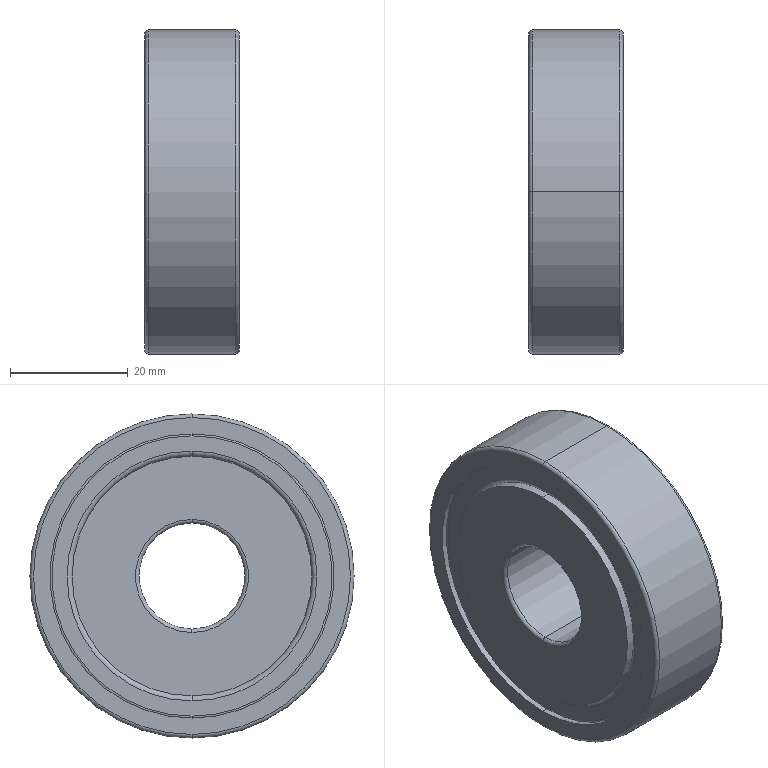Part | STEP file | Completa.sldasm-Part-109_Valor predeterminado | 1 solid | 40 faces | box 16.01 x 55 x 55 mm | volume 32786 mm3 | torus 16 | cylinder 16 | plane 8 | commonest cylinder face diameters 40.7 x4 48.225 x4 49.3 x4 18 x2 55 x2